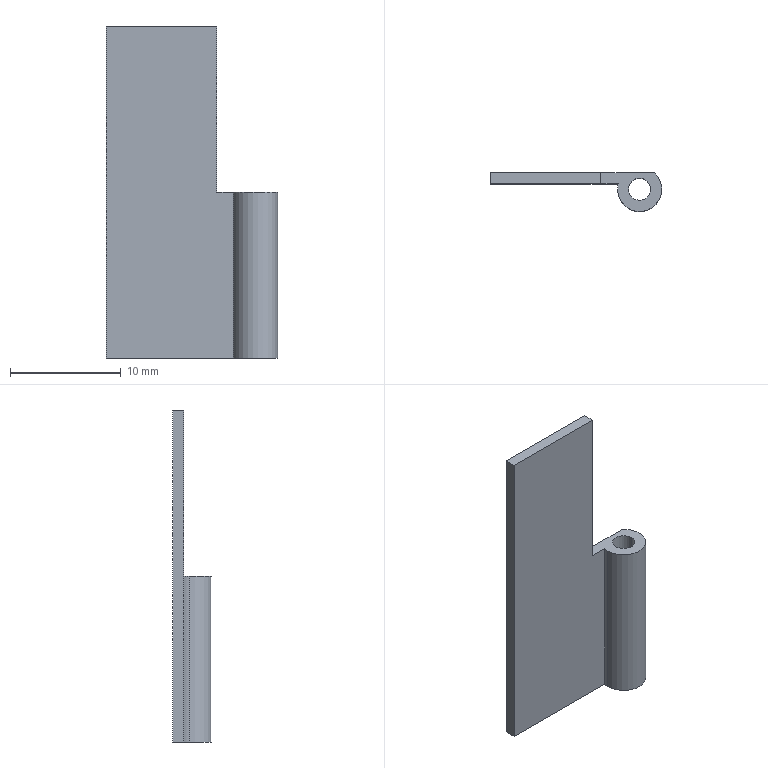Part | STEP file | Hinge leaf 1 | 1 solid | 12 faces | box 15.5 x 3.5 x 30 mm | volume 454.79 mm3 | plane 7 | cylinder 5 | commonest cylinder face diameters 4 x3 2 x2
STEP:
#1=CARTESIAN_POINT('',(0.,0.,0.));
#2=DIRECTION('',(0.,0.,1.));
#3=DIRECTION('',(1.,0.,0.));
#4=AXIS2_PLACEMENT_3D('',#1,#2,#3);
#5=CARTESIAN_POINT('',(15.5,-1.5,15.));
#6=VERTEX_POINT('',#5);
#7=CARTESIAN_POINT('',(14.823,0.,15.));
#8=VERTEX_POINT('',#7);
#9=CARTESIAN_POINT('',(13.5,-1.5,15.));
#10=DIRECTION('',(0.,0.,1.));
#11=DIRECTION('',(-1.,0.,0.));
#12=AXIS2_PLACEMENT_3D('',#9,#10,#11);
#13=CIRCLE('',#12,2.);
#14=CARTESIAN_POINT('',(13.5,-1.5,30.));
#15=DIRECTION('',(0.,0.,-1.));
#16=DIRECTION('',(-1.,0.,0.));
#17=AXIS2_PLACEMENT_3D('',#14,#15,#16);
#18=CYLINDRICAL_SURFACE('',#17,2.);
#19=CARTESIAN_POINT('',(6.283,15.));
#20=DIRECTION('',(-1.,0.));
#21=VECTOR('',#20,1.);
#22=LINE('',#19,#21);
#23=(GEOMETRIC_REPRESENTATION_CONTEXT(2)PARAMETRIC_REPRESENTATION_CONTEXT()REPRESENTATION_CONTEXT('',''));
#24=DEFINITIONAL_REPRESENTATION('',(#22),#23);
#25=PCURVE('',#18,#24);
#26=CARTESIAN_POINT('',(10.,-14.282,15.));
#27=DIRECTION('',(0.,0.,1.));
#28=DIRECTION('',(1.,0.,0.));
#29=AXIS2_PLACEMENT_3D('',#26,#27,#28);
#30=PLANE('',#29);
#31=CARTESIAN_POINT('',(3.5,12.782));
#32=DIRECTION('',(-1.,0.));
#33=AXIS2_PLACEMENT_2D('',#31,#32);
#34=CIRCLE('',#33,2.);
#35=(GEOMETRIC_REPRESENTATION_CONTEXT(2)PARAMETRIC_REPRESENTATION_CONTEXT()REPRESENTATION_CONTEXT('',''));
#36=DEFINITIONAL_REPRESENTATION('',(#34),#35);
#37=PCURVE('',#30,#36);
#38=SURFACE_CURVE('',#13,(#25,#37),.PCURVE_S1.);
#39=EDGE_CURVE('',#6,#8,#38,.T.);
#40=ORIENTED_EDGE('',*,*,#39,.F.);
#41=CARTESIAN_POINT('',(15.5,-1.5,0.));
#42=VERTEX_POINT('',#41);
#43=CARTESIAN_POINT('',(15.5,-1.5,30.));
#44=DIRECTION('',(0.,0.,-1.));
#45=VECTOR('',#44,1.);
#46=LINE('',#43,#45);
#47=CARTESIAN_POINT('',(3.142,0.));
#48=DIRECTION('',(0.,1.));
#49=VECTOR('',#48,1.);
#50=LINE('',#47,#49);
#51=(GEOMETRIC_REPRESENTATION_CONTEXT(2)PARAMETRIC_REPRESENTATION_CONTEXT()REPRESENTATION_CONTEXT('',''));
#52=DEFINITIONAL_REPRESENTATION('',(#50),#51);
#53=PCURVE('',#18,#52);
#54=CARTESIAN_POINT('',(13.5,-1.5,30.));
#55=DIRECTION('',(0.,0.,-1.));
#56=DIRECTION('',(-1.,0.,0.));
#57=AXIS2_PLACEMENT_3D('',#54,#55,#56);
#58=CYLINDRICAL_SURFACE('',#57,2.);
#59=CARTESIAN_POINT('',(3.142,0.));
#60=DIRECTION('',(0.,1.));
#61=VECTOR('',#60,1.);
#62=LINE('',#59,#61);
#63=(GEOMETRIC_REPRESENTATION_CONTEXT(2)PARAMETRIC_REPRESENTATION_CONTEXT()REPRESENTATION_CONTEXT('',''));
#64=DEFINITIONAL_REPRESENTATION('',(#62),#63);
#65=PCURVE('',#58,#64);
#66=SURFACE_CURVE('',#46,(#53,#65),.PCURVE_S1.);
#67=EDGE_CURVE('',#6,#42,#66,.T.);
#68=ORIENTED_EDGE('',*,*,#67,.T.);
#69=CARTESIAN_POINT('',(14.823,0.,0.));
#70=VERTEX_POINT('',#69);
#71=CARTESIAN_POINT('',(13.5,-1.5,0.));
#72=DIRECTION('',(0.,0.,1.));
#73=DIRECTION('',(-1.,0.,0.));
#74=AXIS2_PLACEMENT_3D('',#71,#72,#73);
#75=CIRCLE('',#74,2.);
#76=CARTESIAN_POINT('',(6.283,30.));
#77=DIRECTION('',(-1.,0.));
#78=VECTOR('',#77,1.);
#79=LINE('',#76,#78);
#80=(GEOMETRIC_REPRESENTATION_CONTEXT(2)PARAMETRIC_REPRESENTATION_CONTEXT()REPRESENTATION_CONTEXT('',''));
#81=DEFINITIONAL_REPRESENTATION('',(#79),#80);
#82=PCURVE('',#18,#81);
#83=CARTESIAN_POINT('',(13.5,-1.5,0.));
#84=DIRECTION('',(0.,0.,1.));
#85=DIRECTION('',(1.,0.,0.));
#86=AXIS2_PLACEMENT_3D('',#83,#84,#85);
#87=PLANE('',#86);
#88=CARTESIAN_POINT('',(0.,0.));
#89=DIRECTION('',(-1.,0.));
#90=AXIS2_PLACEMENT_2D('',#88,#89);
#91=CIRCLE('',#90,2.);
#92=(GEOMETRIC_REPRESENTATION_CONTEXT(2)PARAMETRIC_REPRESENTATION_CONTEXT()REPRESENTATION_CONTEXT('',''));
#93=DEFINITIONAL_REPRESENTATION('',(#91),#92);
#94=PCURVE('',#87,#93);
#95=SURFACE_CURVE('',#75,(#82,#94),.PCURVE_S1.);
#96=EDGE_CURVE('',#42,#70,#95,.T.);
#97=ORIENTED_EDGE('',*,*,#96,.T.);
#98=CARTESIAN_POINT('',(14.823,0.,30.));
#99=DIRECTION('',(0.,0.,1.));
#100=VECTOR('',#99,1.);
#101=LINE('',#98,#100);
#102=CARTESIAN_POINT('',(2.294,0.));
#103=DIRECTION('',(0.,-1.));
#104=VECTOR('',#103,1.);
#105=LINE('',#102,#104);
#106=(GEOMETRIC_REPRESENTATION_CONTEXT(2)PARAMETRIC_REPRESENTATION_CONTEXT()REPRESENTATION_CONTEXT('',''));
#107=DEFINITIONAL_REPRESENTATION('',(#105),#106);
#108=PCURVE('',#18,#107);
#109=CARTESIAN_POINT('',(0.,0.,30.));
#110=DIRECTION('',(0.,-1.,0.));
#111=DIRECTION('',(0.,0.,-1.));
#112=AXIS2_PLACEMENT_3D('',#109,#110,#111);
#113=PLANE('',#112);
#114=CARTESIAN_POINT('',(0.,14.823));
#115=DIRECTION('',(-1.,0.));
#116=VECTOR('',#115,1.);
#117=LINE('',#114,#116);
#118=(GEOMETRIC_REPRESENTATION_CONTEXT(2)PARAMETRIC_REPRESENTATION_CONTEXT()REPRESENTATION_CONTEXT('',''));
#119=DEFINITIONAL_REPRESENTATION('',(#117),#118);
#120=PCURVE('',#113,#119);
#121=SURFACE_CURVE('',#101,(#108,#120),.PCURVE_S1.);
#122=EDGE_CURVE('',#70,#8,#121,.T.);
#123=ORIENTED_EDGE('',*,*,#122,.T.);
#124=EDGE_LOOP('',(#40,#68,#97,#123));
#125=FACE_BOUND('',#124,.T.);
#126=ADVANCED_FACE('',(#125),#18,.T.);
#127=ORIENTED_EDGE('',*,*,#67,.F.);
#128=CARTESIAN_POINT('',(11.5,-1.5,15.));
#129=VERTEX_POINT('',#128);
#130=CARTESIAN_POINT('',(13.5,-1.5,15.));
#131=DIRECTION('',(0.,0.,1.));
#132=DIRECTION('',(-1.,0.,0.));
#133=AXIS2_PLACEMENT_3D('',#130,#131,#132);
#134=CIRCLE('',#133,2.);
#135=CARTESIAN_POINT('',(6.283,15.));
#136=DIRECTION('',(-1.,0.));
#137=VECTOR('',#136,1.);
#138=LINE('',#135,#137);
#139=(GEOMETRIC_REPRESENTATION_CONTEXT(2)PARAMETRIC_REPRESENTATION_CONTEXT()REPRESENTATION_CONTEXT('',''));
#140=DEFINITIONAL_REPRESENTATION('',(#138),#139);
#141=PCURVE('',#58,#140);
#142=CARTESIAN_POINT('',(3.5,12.782));
#143=DIRECTION('',(-1.,0.));
#144=AXIS2_PLACEMENT_2D('',#142,#143);
#145=CIRCLE('',#144,2.);
#146=(GEOMETRIC_REPRESENTATION_CONTEXT(2)PARAMETRIC_REPRESENTATION_CONTEXT()REPRESENTATION_CONTEXT('',''));
#147=DEFINITIONAL_REPRESENTATION('',(#145),#146);
#148=PCURVE('',#30,#147);
#149=SURFACE_CURVE('',#134,(#141,#148),.PCURVE_S1.);
#150=EDGE_CURVE('',#129,#6,#149,.T.);
#151=ORIENTED_EDGE('',*,*,#150,.F.);
#152=CARTESIAN_POINT('',(11.5,-1.5,0.));
#153=VERTEX_POINT('',#152);
#154=CARTESIAN_POINT('',(11.5,-1.5,30.));
#155=DIRECTION('',(0.,0.,-1.));
#156=VECTOR('',#155,1.);
#157=LINE('',#154,#156);
#158=CARTESIAN_POINT('',(6.283,0.));
#159=DIRECTION('',(0.,1.));
#160=VECTOR('',#159,1.);
#161=LINE('',#158,#160);
#162=(GEOMETRIC_REPRESENTATION_CONTEXT(2)PARAMETRIC_REPRESENTATION_CONTEXT()REPRESENTATION_CONTEXT('',''));
#163=DEFINITIONAL_REPRESENTATION('',(#161),#162);
#164=PCURVE('',#58,#163);
#165=CARTESIAN_POINT('',(13.5,-1.5,30.));
#166=DIRECTION('',(0.,0.,-1.));
#167=DIRECTION('',(-1.,0.,0.));
#168=AXIS2_PLACEMENT_3D('',#165,#166,#167);
#169=CYLINDRICAL_SURFACE('',#168,2.);
#170=CARTESIAN_POINT('',(0.,0.));
#171=DIRECTION('',(0.,1.));
#172=VECTOR('',#171,1.);
#173=LINE('',#170,#172);
#174=(GEOMETRIC_REPRESENTATION_CONTEXT(2)PARAMETRIC_REPRESENTATION_CONTEXT()REPRESENTATION_CONTEXT('',''));
#175=DEFINITIONAL_REPRESENTATION('',(#173),#174);
#176=PCURVE('',#169,#175);
#177=SURFACE_CURVE('',#157,(#164,#176),.PCURVE_S1.);
#178=EDGE_CURVE('',#129,#153,#177,.T.);
#179=ORIENTED_EDGE('',*,*,#178,.T.);
#180=CARTESIAN_POINT('',(13.5,-1.5,0.));
#181=DIRECTION('',(0.,0.,1.));
#182=DIRECTION('',(-1.,0.,0.));
#183=AXIS2_PLACEMENT_3D('',#180,#181,#182);
#184=CIRCLE('',#183,2.);
#185=CARTESIAN_POINT('',(6.283,30.));
#186=DIRECTION('',(-1.,0.));
#187=VECTOR('',#186,1.);
#188=LINE('',#185,#187);
#189=(GEOMETRIC_REPRESENTATION_CONTEXT(2)PARAMETRIC_REPRESENTATION_CONTEXT()REPRESENTATION_CONTEXT('',''));
#190=DEFINITIONAL_REPRESENTATION('',(#188),#189);
#191=PCURVE('',#58,#190);
#192=CARTESIAN_POINT('',(0.,0.));
#193=DIRECTION('',(-1.,0.));
#194=AXIS2_PLACEMENT_2D('',#192,#193);
#195=CIRCLE('',#194,2.);
#196=(GEOMETRIC_REPRESENTATION_CONTEXT(2)PARAMETRIC_REPRESENTATION_CONTEXT()REPRESENTATION_CONTEXT('',''));
#197=DEFINITIONAL_REPRESENTATION('',(#195),#196);
#198=PCURVE('',#87,#197);
#199=SURFACE_CURVE('',#184,(#191,#198),.PCURVE_S1.);
#200=EDGE_CURVE('',#153,#42,#199,.T.);
#201=ORIENTED_EDGE('',*,*,#200,.T.);
#202=EDGE_LOOP('',(#127,#151,#179,#201));
#203=FACE_BOUND('',#202,.T.);
#204=ADVANCED_FACE('',(#203),#58,.T.);
#205=CARTESIAN_POINT('',(12.5,-1.5,15.));
#206=VERTEX_POINT('',#205);
#207=CARTESIAN_POINT('',(12.5,-1.5,0.));
#208=VERTEX_POINT('',#207);
#209=CARTESIAN_POINT('',(12.5,-1.5,30.));
#210=DIRECTION('',(0.,0.,-1.));
#211=VECTOR('',#210,1.);
#212=LINE('',#209,#211);
#213=CARTESIAN_POINT('',(13.5,-1.5,30.));
#214=DIRECTION('',(0.,0.,-1.));
#215=DIRECTION('',(-1.,0.,0.));
#216=AXIS2_PLACEMENT_3D('',#213,#214,#215);
#217=CYLINDRICAL_SURFACE('',#216,1.);
#218=CARTESIAN_POINT('',(6.283,0.));
#219=DIRECTION('',(0.,1.));
#220=VECTOR('',#219,1.);
#221=LINE('',#218,#220);
#222=(GEOMETRIC_REPRESENTATION_CONTEXT(2)PARAMETRIC_REPRESENTATION_CONTEXT()REPRESENTATION_CONTEXT('',''));
#223=DEFINITIONAL_REPRESENTATION('',(#221),#222);
#224=PCURVE('',#217,#223);
#225=CARTESIAN_POINT('',(13.5,-1.5,30.));
#226=DIRECTION('',(0.,0.,-1.));
#227=DIRECTION('',(-1.,0.,0.));
#228=AXIS2_PLACEMENT_3D('',#225,#226,#227);
#229=CYLINDRICAL_SURFACE('',#228,1.);
#230=CARTESIAN_POINT('',(0.,0.));
#231=DIRECTION('',(0.,1.));
#232=VECTOR('',#231,1.);
#233=LINE('',#230,#232);
#234=(GEOMETRIC_REPRESENTATION_CONTEXT(2)PARAMETRIC_REPRESENTATION_CONTEXT()REPRESENTATION_CONTEXT('',''));
#235=DEFINITIONAL_REPRESENTATION('',(#233),#234);
#236=PCURVE('',#229,#235);
#237=SURFACE_CURVE('',#212,(#224,#236),.PCURVE_S1.);
#238=EDGE_CURVE('',#206,#208,#237,.T.);
#239=ORIENTED_EDGE('',*,*,#238,.T.);
#240=CARTESIAN_POINT('',(14.5,-1.5,0.));
#241=VERTEX_POINT('',#240);
#242=CARTESIAN_POINT('',(13.5,-1.5,0.));
#243=DIRECTION('',(0.,0.,-1.));
#244=DIRECTION('',(-1.,0.,0.));
#245=AXIS2_PLACEMENT_3D('',#242,#243,#244);
#246=CIRCLE('',#245,1.);
#247=CARTESIAN_POINT('',(0.,30.));
#248=DIRECTION('',(1.,0.));
#249=VECTOR('',#248,1.);
#250=LINE('',#247,#249);
#251=(GEOMETRIC_REPRESENTATION_CONTEXT(2)PARAMETRIC_REPRESENTATION_CONTEXT()REPRESENTATION_CONTEXT('',''));
#252=DEFINITIONAL_REPRESENTATION('',(#250),#251);
#253=PCURVE('',#217,#252);
#254=CARTESIAN_POINT('',(-1.,0.));
#255=CARTESIAN_POINT('',(-1.,1.732));
#256=CARTESIAN_POINT('',(0.5,0.866));
#257=CARTESIAN_POINT('',(2.,0.));
#258=CARTESIAN_POINT('',(0.5,-0.866));
#259=CARTESIAN_POINT('',(-1.,-1.732));
#260=CARTESIAN_POINT('',(-1.,0.));
#261=(BOUNDED_CURVE()B_SPLINE_CURVE(2,(#254,#255,#256,#257,#258,#259,#260),.UNSPECIFIED.,.T.,.F.)B_SPLINE_CURVE_WITH_KNOTS((1,2,2,2,2,1),(-2.094,0.,2.094,4.189,6.283,8.378),.UNSPECIFIED.)CURVE()GEOMETRIC_REPRESENTATION_ITEM()RATIONAL_B_SPLINE_CURVE((1.,0.5,1.,0.5,1.,0.5,1.))REPRESENTATION_ITEM(''));
#262=(GEOMETRIC_REPRESENTATION_CONTEXT(2)PARAMETRIC_REPRESENTATION_CONTEXT()REPRESENTATION_CONTEXT('',''));
#263=DEFINITIONAL_REPRESENTATION('',(#261),#262);
#264=PCURVE('',#87,#263);
#265=SURFACE_CURVE('',#246,(#253,#264),.PCURVE_S1.);
#266=EDGE_CURVE('',#241,#208,#265,.T.);
#267=ORIENTED_EDGE('',*,*,#266,.F.);
#268=CARTESIAN_POINT('',(14.5,-1.5,15.));
#269=VERTEX_POINT('',#268);
#270=CARTESIAN_POINT('',(14.5,-1.5,30.));
#271=DIRECTION('',(0.,0.,-1.));
#272=VECTOR('',#271,1.);
#273=LINE('',#270,#272);
#274=CARTESIAN_POINT('',(3.142,0.));
#275=DIRECTION('',(0.,1.));
#276=VECTOR('',#275,1.);
#277=LINE('',#274,#276);
#278=(GEOMETRIC_REPRESENTATION_CONTEXT(2)PARAMETRIC_REPRESENTATION_CONTEXT()REPRESENTATION_CONTEXT('',''));
#279=DEFINITIONAL_REPRESENTATION('',(#277),#278);
#280=PCURVE('',#217,#279);
#281=CARTESIAN_POINT('',(3.142,0.));
#282=DIRECTION('',(0.,1.));
#283=VECTOR('',#282,1.);
#284=LINE('',#281,#283);
#285=(GEOMETRIC_REPRESENTATION_CONTEXT(2)PARAMETRIC_REPRESENTATION_CONTEXT()REPRESENTATION_CONTEXT('',''));
#286=DEFINITIONAL_REPRESENTATION('',(#284),#285);
#287=PCURVE('',#229,#286);
#288=SURFACE_CURVE('',#273,(#280,#287),.PCURVE_S1.);
#289=EDGE_CURVE('',#269,#241,#288,.T.);
#290=ORIENTED_EDGE('',*,*,#289,.F.);
#291=CARTESIAN_POINT('',(13.5,-1.5,15.));
#292=DIRECTION('',(0.,0.,-1.));
#293=DIRECTION('',(-1.,0.,0.));
#294=AXIS2_PLACEMENT_3D('',#291,#292,#293);
#295=CIRCLE('',#294,1.);
#296=CARTESIAN_POINT('',(0.,15.));
#297=DIRECTION('',(1.,0.));
#298=VECTOR('',#297,1.);
#299=LINE('',#296,#298);
#300=(GEOMETRIC_REPRESENTATION_CONTEXT(2)PARAMETRIC_REPRESENTATION_CONTEXT()REPRESENTATION_CONTEXT('',''));
#301=DEFINITIONAL_REPRESENTATION('',(#299),#300);
#302=PCURVE('',#217,#301);
#303=CARTESIAN_POINT('',(2.5,12.782));
#304=CARTESIAN_POINT('',(2.5,14.514));
#305=CARTESIAN_POINT('',(4.,13.648));
#306=CARTESIAN_POINT('',(5.5,12.782));
#307=CARTESIAN_POINT('',(4.,11.916));
#308=CARTESIAN_POINT('',(2.5,11.05));
#309=CARTESIAN_POINT('',(2.5,12.782));
#310=(BOUNDED_CURVE()B_SPLINE_CURVE(2,(#303,#304,#305,#306,#307,#308,#309),.UNSPECIFIED.,.T.,.F.)B_SPLINE_CURVE_WITH_KNOTS((1,2,2,2,2,1),(-2.094,0.,2.094,4.189,6.283,8.378),.UNSPECIFIED.)CURVE()GEOMETRIC_REPRESENTATION_ITEM()RATIONAL_B_SPLINE_CURVE((1.,0.5,1.,0.5,1.,0.5,1.))REPRESENTATION_ITEM(''));
#311=(GEOMETRIC_REPRESENTATION_CONTEXT(2)PARAMETRIC_REPRESENTATION_CONTEXT()REPRESENTATION_CONTEXT('',''));
#312=DEFINITIONAL_REPRESENTATION('',(#310),#311);
#313=PCURVE('',#30,#312);
#314=SURFACE_CURVE('',#295,(#302,#313),.PCURVE_S1.);
#315=EDGE_CURVE('',#269,#206,#314,.T.);
#316=ORIENTED_EDGE('',*,*,#315,.T.);
#317=EDGE_LOOP('',(#239,#267,#290,#316));
#318=FACE_BOUND('',#317,.F.);
#319=ADVANCED_FACE('',(#318),#217,.F.);
#320=CARTESIAN_POINT('',(10.,0.,15.));
#321=VERTEX_POINT('',#320);
#322=CARTESIAN_POINT('',(10.,0.,30.));
#323=VERTEX_POINT('',#322);
#324=CARTESIAN_POINT('',(10.,0.,30.));
#325=DIRECTION('',(0.,0.,1.));
#326=VECTOR('',#325,1.);
#327=LINE('',#324,#326);
#328=CARTESIAN_POINT('',(0.,10.));
#329=DIRECTION('',(-1.,0.));
#330=VECTOR('',#329,1.);
#331=LINE('',#328,#330);
#332=(GEOMETRIC_REPRESENTATION_CONTEXT(2)PARAMETRIC_REPRESENTATION_CONTEXT()REPRESENTATION_CONTEXT('',''));
#333=DEFINITIONAL_REPRESENTATION('',(#331),#332);
#334=PCURVE('',#113,#333);
#335=CARTESIAN_POINT('',(10.,2.063,15.));
#336=DIRECTION('',(-1.,0.,0.));
#337=DIRECTION('',(0.,-1.,0.));
#338=AXIS2_PLACEMENT_3D('',#335,#336,#337);
#339=PLANE('',#338);
#340=CARTESIAN_POINT('',(2.063,15.));
#341=DIRECTION('',(0.,1.));
#342=VECTOR('',#341,1.);
#343=LINE('',#340,#342);
#344=(GEOMETRIC_REPRESENTATION_CONTEXT(2)PARAMETRIC_REPRESENTATION_CONTEXT()REPRESENTATION_CONTEXT('',''));
#345=DEFINITIONAL_REPRESENTATION('',(#343),#344);
#346=PCURVE('',#339,#345);
#347=SURFACE_CURVE('',#327,(#334,#346),.PCURVE_S1.);
#348=EDGE_CURVE('',#321,#323,#347,.T.);
#349=ORIENTED_EDGE('',*,*,#348,.F.);
#350=CARTESIAN_POINT('',(0.,0.,15.));
#351=DIRECTION('',(-1.,0.,0.));
#352=VECTOR('',#351,1.);
#353=LINE('',#350,#352);
#354=CARTESIAN_POINT('',(15.,0.));
#355=DIRECTION('',(0.,-1.));
#356=VECTOR('',#355,1.);
#357=LINE('',#354,#356);
#358=(GEOMETRIC_REPRESENTATION_CONTEXT(2)PARAMETRIC_REPRESENTATION_CONTEXT()REPRESENTATION_CONTEXT('',''));
#359=DEFINITIONAL_REPRESENTATION('',(#357),#358);
#360=PCURVE('',#113,#359);
#361=CARTESIAN_POINT('',(-10.,14.282));
#362=DIRECTION('',(-1.,0.));
#363=VECTOR('',#362,1.);
#364=LINE('',#361,#363);
#365=(GEOMETRIC_REPRESENTATION_CONTEXT(2)PARAMETRIC_REPRESENTATION_CONTEXT()REPRESENTATION_CONTEXT('',''));
#366=DEFINITIONAL_REPRESENTATION('',(#364),#365);
#367=PCURVE('',#30,#366);
#368=SURFACE_CURVE('',#353,(#360,#367),.PCURVE_S1.);
#369=EDGE_CURVE('',#8,#321,#368,.T.);
#370=ORIENTED_EDGE('',*,*,#369,.F.);
#371=ORIENTED_EDGE('',*,*,#122,.F.);
#372=CARTESIAN_POINT('',(0.,0.,0.));
#373=VERTEX_POINT('',#372);
#374=CARTESIAN_POINT('',(0.,0.,0.));
#375=DIRECTION('',(1.,0.,0.));
#376=VECTOR('',#375,1.);
#377=LINE('',#374,#376);
#378=CARTESIAN_POINT('',(30.,0.));
#379=DIRECTION('',(0.,1.));
#380=VECTOR('',#379,1.);
#381=LINE('',#378,#380);
#382=(GEOMETRIC_REPRESENTATION_CONTEXT(2)PARAMETRIC_REPRESENTATION_CONTEXT()REPRESENTATION_CONTEXT('',''));
#383=DEFINITIONAL_REPRESENTATION('',(#381),#382);
#384=PCURVE('',#113,#383);
#385=CARTESIAN_POINT('',(-13.5,1.5));
#386=DIRECTION('',(1.,0.));
#387=VECTOR('',#386,1.);
#388=LINE('',#385,#387);
#389=(GEOMETRIC_REPRESENTATION_CONTEXT(2)PARAMETRIC_REPRESENTATION_CONTEXT()REPRESENTATION_CONTEXT('',''));
#390=DEFINITIONAL_REPRESENTATION('',(#388),#389);
#391=PCURVE('',#87,#390);
#392=SURFACE_CURVE('',#377,(#384,#391),.PCURVE_S1.);
#393=EDGE_CURVE('',#373,#70,#392,.T.);
#394=ORIENTED_EDGE('',*,*,#393,.F.);
#395=CARTESIAN_POINT('',(0.,0.,30.));
#396=VERTEX_POINT('',#395);
#397=CARTESIAN_POINT('',(0.,0.,30.));
#398=DIRECTION('',(0.,0.,-1.));
#399=VECTOR('',#398,1.);
#400=LINE('',#397,#399);
#401=CARTESIAN_POINT('',(0.,0.));
#402=DIRECTION('',(1.,0.));
#403=VECTOR('',#402,1.);
#404=LINE('',#401,#403);
#405=(GEOMETRIC_REPRESENTATION_CONTEXT(2)PARAMETRIC_REPRESENTATION_CONTEXT()REPRESENTATION_CONTEXT('',''));
#406=DEFINITIONAL_REPRESENTATION('',(#404),#405);
#407=PCURVE('',#113,#406);
#408=CARTESIAN_POINT('',(0.,0.,30.));
#409=DIRECTION('',(1.,0.,0.));
#410=DIRECTION('',(0.,1.,0.));
#411=AXIS2_PLACEMENT_3D('',#408,#409,#410);
#412=PLANE('',#411);
#413=CARTESIAN_POINT('',(0.,0.));
#414=DIRECTION('',(0.,-1.));
#415=VECTOR('',#414,1.);
#416=LINE('',#413,#415);
#417=(GEOMETRIC_REPRESENTATION_CONTEXT(2)PARAMETRIC_REPRESENTATION_CONTEXT()REPRESENTATION_CONTEXT('',''));
#418=DEFINITIONAL_REPRESENTATION('',(#416),#417);
#419=PCURVE('',#412,#418);
#420=SURFACE_CURVE('',#400,(#407,#419),.PCURVE_S1.);
#421=EDGE_CURVE('',#396,#373,#420,.T.);
#422=ORIENTED_EDGE('',*,*,#421,.F.);
#423=CARTESIAN_POINT('',(0.,0.,30.));
#424=DIRECTION('',(-1.,0.,0.));
#425=VECTOR('',#424,1.);
#426=LINE('',#423,#425);
#427=CARTESIAN_POINT('',(0.,0.));
#428=DIRECTION('',(0.,-1.));
#429=VECTOR('',#428,1.);
#430=LINE('',#427,#429);
#431=(GEOMETRIC_REPRESENTATION_CONTEXT(2)PARAMETRIC_REPRESENTATION_CONTEXT()REPRESENTATION_CONTEXT('',''));
#432=DEFINITIONAL_REPRESENTATION('',(#430),#431);
#433=PCURVE('',#113,#432);
#434=CARTESIAN_POINT('',(13.5,-1.5,30.));
#435=DIRECTION('',(0.,0.,1.));
#436=DIRECTION('',(1.,0.,0.));
#437=AXIS2_PLACEMENT_3D('',#434,#435,#436);
#438=PLANE('',#437);
#439=CARTESIAN_POINT('',(-13.5,1.5));
#440=DIRECTION('',(-1.,0.));
#441=VECTOR('',#440,1.);
#442=LINE('',#439,#441);
#443=(GEOMETRIC_REPRESENTATION_CONTEXT(2)PARAMETRIC_REPRESENTATION_CONTEXT()REPRESENTATION_CONTEXT('',''));
#444=DEFINITIONAL_REPRESENTATION('',(#442),#443);
#445=PCURVE('',#438,#444);
#446=SURFACE_CURVE('',#426,(#433,#445),.PCURVE_S1.);
#447=EDGE_CURVE('',#323,#396,#446,.T.);
#448=ORIENTED_EDGE('',*,*,#447,.F.);
#449=EDGE_LOOP('',(#349,#370,#371,#394,#422,#448));
#450=FACE_BOUND('',#449,.T.);
#451=ADVANCED_FACE('',(#450),#113,.F.);
#452=CARTESIAN_POINT('',(0.,-1.,30.));
#453=VERTEX_POINT('',#452);
#454=CARTESIAN_POINT('',(0.,-1.5,30.));
#455=DIRECTION('',(0.,-1.,0.));
#456=VECTOR('',#455,1.);
#457=LINE('',#454,#456);
#458=CARTESIAN_POINT('',(-13.5,0.));
#459=DIRECTION('',(0.,-1.));
#460=VECTOR('',#459,1.);
#461=LINE('',#458,#460);
#462=(GEOMETRIC_REPRESENTATION_CONTEXT(2)PARAMETRIC_REPRESENTATION_CONTEXT()REPRESENTATION_CONTEXT('',''));
#463=DEFINITIONAL_REPRESENTATION('',(#461),#462);
#464=PCURVE('',#438,#463);
#465=CARTESIAN_POINT('',(-1.5,0.));
#466=DIRECTION('',(-1.,0.));
#467=VECTOR('',#466,1.);
#468=LINE('',#465,#467);
#469=(GEOMETRIC_REPRESENTATION_CONTEXT(2)PARAMETRIC_REPRESENTATION_CONTEXT()REPRESENTATION_CONTEXT('',''));
#470=DEFINITIONAL_REPRESENTATION('',(#468),#469);
#471=PCURVE('',#412,#470);
#472=SURFACE_CURVE('',#457,(#464,#471),.PCURVE_S1.);
#473=EDGE_CURVE('',#396,#453,#472,.T.);
#474=ORIENTED_EDGE('',*,*,#473,.T.);
#475=CARTESIAN_POINT('',(10.,-1.,30.));
#476=VERTEX_POINT('',#475);
#477=CARTESIAN_POINT('',(13.5,-1.,30.));
#478=DIRECTION('',(1.,0.,0.));
#479=VECTOR('',#478,1.);
#480=LINE('',#477,#479);
#481=CARTESIAN_POINT('',(0.,0.5));
#482=DIRECTION('',(1.,0.));
#483=VECTOR('',#482,1.);
#484=LINE('',#481,#483);
#485=(GEOMETRIC_REPRESENTATION_CONTEXT(2)PARAMETRIC_REPRESENTATION_CONTEXT()REPRESENTATION_CONTEXT('',''));
#486=DEFINITIONAL_REPRESENTATION('',(#484),#485);
#487=PCURVE('',#438,#486);
#488=CARTESIAN_POINT('',(0.,-1.,30.));
#489=DIRECTION('',(0.,1.,0.));
#490=DIRECTION('',(-1.,0.,0.));
#491=AXIS2_PLACEMENT_3D('',#488,#489,#490);
#492=PLANE('',#491);
#493=CARTESIAN_POINT('',(-13.5,0.));
#494=DIRECTION('',(-1.,0.));
#495=VECTOR('',#494,1.);
#496=LINE('',#493,#495);
#497=(GEOMETRIC_REPRESENTATION_CONTEXT(2)PARAMETRIC_REPRESENTATION_CONTEXT()REPRESENTATION_CONTEXT('',''));
#498=DEFINITIONAL_REPRESENTATION('',(#496),#497);
#499=PCURVE('',#492,#498);
#500=SURFACE_CURVE('',#480,(#487,#499),.PCURVE_S1.);
#501=EDGE_CURVE('',#453,#476,#500,.T.);
#502=ORIENTED_EDGE('',*,*,#501,.T.);
#503=CARTESIAN_POINT('',(10.,-1.5,30.));
#504=DIRECTION('',(0.,1.,0.));
#505=VECTOR('',#504,1.);
#506=LINE('',#503,#505);
#507=CARTESIAN_POINT('',(-3.5,0.));
#508=DIRECTION('',(0.,1.));
#509=VECTOR('',#508,1.);
#510=LINE('',#507,#509);
#511=(GEOMETRIC_REPRESENTATION_CONTEXT(2)PARAMETRIC_REPRESENTATION_CONTEXT()REPRESENTATION_CONTEXT('',''));
#512=DEFINITIONAL_REPRESENTATION('',(#510),#511);
#513=PCURVE('',#438,#512);
#514=CARTESIAN_POINT('',(3.563,15.));
#515=DIRECTION('',(-1.,0.));
#516=VECTOR('',#515,1.);
#517=LINE('',#514,#516);
#518=(GEOMETRIC_REPRESENTATION_CONTEXT(2)PARAMETRIC_REPRESENTATION_CONTEXT()REPRESENTATION_CONTEXT('',''));
#519=DEFINITIONAL_REPRESENTATION('',(#517),#518);
#520=PCURVE('',#339,#519);
#521=SURFACE_CURVE('',#506,(#513,#520),.PCURVE_S1.);
#522=EDGE_CURVE('',#476,#323,#521,.T.);
#523=ORIENTED_EDGE('',*,*,#522,.T.);
#524=ORIENTED_EDGE('',*,*,#447,.T.);
#525=EDGE_LOOP('',(#474,#502,#523,#524));
#526=FACE_BOUND('',#525,.T.);
#527=ADVANCED_FACE('',(#526),#438,.T.);
#528=CARTESIAN_POINT('',(10.,-1.,15.));
#529=VERTEX_POINT('',#528);
#530=CARTESIAN_POINT('',(10.,-1.,15.));
#531=DIRECTION('',(0.,0.,1.));
#532=VECTOR('',#531,1.);
#533=LINE('',#530,#532);
#534=CARTESIAN_POINT('',(3.063,0.));
#535=DIRECTION('',(0.,1.));
#536=VECTOR('',#535,1.);
#537=LINE('',#534,#536);
#538=(GEOMETRIC_REPRESENTATION_CONTEXT(2)PARAMETRIC_REPRESENTATION_CONTEXT()REPRESENTATION_CONTEXT('',''));
#539=DEFINITIONAL_REPRESENTATION('',(#537),#538);
#540=PCURVE('',#339,#539);
#541=CARTESIAN_POINT('',(-10.,-15.));
#542=DIRECTION('',(0.,1.));
#543=VECTOR('',#542,1.);
#544=LINE('',#541,#543);
#545=(GEOMETRIC_REPRESENTATION_CONTEXT(2)PARAMETRIC_REPRESENTATION_CONTEXT()REPRESENTATION_CONTEXT('',''));
#546=DEFINITIONAL_REPRESENTATION('',(#544),#545);
#547=PCURVE('',#492,#546);
#548=SURFACE_CURVE('',#533,(#540,#547),.PCURVE_S1.);
#549=EDGE_CURVE('',#529,#476,#548,.T.);
#550=ORIENTED_EDGE('',*,*,#549,.F.);
#551=CARTESIAN_POINT('',(10.,2.063,15.));
#552=DIRECTION('',(0.,-1.,0.));
#553=VECTOR('',#552,1.);
#554=LINE('',#551,#553);
#555=CARTESIAN_POINT('',(0.,0.));
#556=DIRECTION('',(1.,0.));
#557=VECTOR('',#556,1.);
#558=LINE('',#555,#557);
#559=(GEOMETRIC_REPRESENTATION_CONTEXT(2)PARAMETRIC_REPRESENTATION_CONTEXT()REPRESENTATION_CONTEXT('',''));
#560=DEFINITIONAL_REPRESENTATION('',(#558),#559);
#561=PCURVE('',#339,#560);
#562=CARTESIAN_POINT('',(0.,16.345));
#563=DIRECTION('',(0.,-1.));
#564=VECTOR('',#563,1.);
#565=LINE('',#562,#564);
#566=(GEOMETRIC_REPRESENTATION_CONTEXT(2)PARAMETRIC_REPRESENTATION_CONTEXT()REPRESENTATION_CONTEXT('',''));
#567=DEFINITIONAL_REPRESENTATION('',(#565),#566);
#568=PCURVE('',#30,#567);
#569=SURFACE_CURVE('',#554,(#561,#568),.PCURVE_S1.);
#570=EDGE_CURVE('',#321,#529,#569,.T.);
#571=ORIENTED_EDGE('',*,*,#570,.F.);
#572=ORIENTED_EDGE('',*,*,#348,.T.);
#573=ORIENTED_EDGE('',*,*,#522,.F.);
#574=EDGE_LOOP('',(#550,#571,#572,#573));
#575=FACE_BOUND('',#574,.T.);
#576=ADVANCED_FACE('',(#575),#339,.F.);
#577=CARTESIAN_POINT('',(11.564,-1.,15.));
#578=VERTEX_POINT('',#577);
#579=CARTESIAN_POINT('',(10.,-1.,15.));
#580=DIRECTION('',(1.,0.,0.));
#581=VECTOR('',#580,1.);
#582=LINE('',#579,#581);
#583=CARTESIAN_POINT('',(0.,13.282));
#584=DIRECTION('',(1.,0.));
#585=VECTOR('',#584,1.);
#586=LINE('',#583,#585);
#587=(GEOMETRIC_REPRESENTATION_CONTEXT(2)PARAMETRIC_REPRESENTATION_CONTEXT()REPRESENTATION_CONTEXT('',''));
#588=DEFINITIONAL_REPRESENTATION('',(#586),#587);
#589=PCURVE('',#30,#588);
#590=CARTESIAN_POINT('',(-10.,-15.));
#591=DIRECTION('',(-1.,0.));
#592=VECTOR('',#591,1.);
#593=LINE('',#590,#592);
#594=(GEOMETRIC_REPRESENTATION_CONTEXT(2)PARAMETRIC_REPRESENTATION_CONTEXT()REPRESENTATION_CONTEXT('',''));
#595=DEFINITIONAL_REPRESENTATION('',(#593),#594);
#596=PCURVE('',#492,#595);
#597=SURFACE_CURVE('',#582,(#589,#596),.PCURVE_S1.);
#598=EDGE_CURVE('',#529,#578,#597,.T.);
#599=ORIENTED_EDGE('',*,*,#598,.T.);
#600=CARTESIAN_POINT('',(13.5,-1.5,15.));
#601=DIRECTION('',(0.,0.,1.));
#602=DIRECTION('',(-1.,0.,0.));
#603=AXIS2_PLACEMENT_3D('',#600,#601,#602);
#604=CIRCLE('',#603,2.);
#605=CARTESIAN_POINT('',(3.5,12.782));
#606=DIRECTION('',(-1.,0.));
#607=AXIS2_PLACEMENT_2D('',#605,#606);
#608=CIRCLE('',#607,2.);
#609=(GEOMETRIC_REPRESENTATION_CONTEXT(2)PARAMETRIC_REPRESENTATION_CONTEXT()REPRESENTATION_CONTEXT('',''));
#610=DEFINITIONAL_REPRESENTATION('',(#608),#609);
#611=PCURVE('',#30,#610);
#612=CARTESIAN_POINT('',(6.283,15.));
#613=DIRECTION('',(-1.,0.));
#614=VECTOR('',#613,1.);
#615=LINE('',#612,#614);
#616=(GEOMETRIC_REPRESENTATION_CONTEXT(2)PARAMETRIC_REPRESENTATION_CONTEXT()REPRESENTATION_CONTEXT('',''));
#617=DEFINITIONAL_REPRESENTATION('',(#615),#616);
#618=PCURVE('',#169,#617);
#619=SURFACE_CURVE('',#604,(#611,#618),.PCURVE_S1.);
#620=EDGE_CURVE('',#578,#129,#619,.T.);
#621=ORIENTED_EDGE('',*,*,#620,.T.);
#622=ORIENTED_EDGE('',*,*,#150,.T.);
#623=ORIENTED_EDGE('',*,*,#39,.T.);
#624=ORIENTED_EDGE('',*,*,#369,.T.);
#625=ORIENTED_EDGE('',*,*,#570,.T.);
#626=EDGE_LOOP('',(#599,#621,#622,#623,#624,#625));
#627=FACE_BOUND('',#626,.T.);
#628=CARTESIAN_POINT('',(13.5,-1.5,15.));
#629=DIRECTION('',(0.,0.,-1.));
#630=DIRECTION('',(-1.,0.,0.));
#631=AXIS2_PLACEMENT_3D('',#628,#629,#630);
#632=CIRCLE('',#631,1.);
#633=CARTESIAN_POINT('',(2.5,12.782));
#634=CARTESIAN_POINT('',(2.5,14.514));
#635=CARTESIAN_POINT('',(4.,13.648));
#636=CARTESIAN_POINT('',(5.5,12.782));
#637=CARTESIAN_POINT('',(4.,11.916));
#638=CARTESIAN_POINT('',(2.5,11.05));
#639=CARTESIAN_POINT('',(2.5,12.782));
#640=(BOUNDED_CURVE()B_SPLINE_CURVE(2,(#633,#634,#635,#636,#637,#638,#639),.UNSPECIFIED.,.T.,.F.)B_SPLINE_CURVE_WITH_KNOTS((1,2,2,2,2,1),(-2.094,0.,2.094,4.189,6.283,8.378),.UNSPECIFIED.)CURVE()GEOMETRIC_REPRESENTATION_ITEM()RATIONAL_B_SPLINE_CURVE((1.,0.5,1.,0.5,1.,0.5,1.))REPRESENTATION_ITEM(''));
#641=(GEOMETRIC_REPRESENTATION_CONTEXT(2)PARAMETRIC_REPRESENTATION_CONTEXT()REPRESENTATION_CONTEXT('',''));
#642=DEFINITIONAL_REPRESENTATION('',(#640),#641);
#643=PCURVE('',#30,#642);
#644=CARTESIAN_POINT('',(0.,15.));
#645=DIRECTION('',(1.,0.));
#646=VECTOR('',#645,1.);
#647=LINE('',#644,#646);
#648=(GEOMETRIC_REPRESENTATION_CONTEXT(2)PARAMETRIC_REPRESENTATION_CONTEXT()REPRESENTATION_CONTEXT('',''));
#649=DEFINITIONAL_REPRESENTATION('',(#647),#648);
#650=PCURVE('',#229,#649);
#651=SURFACE_CURVE('',#632,(#643,#650),.PCURVE_S1.);
#652=EDGE_CURVE('',#206,#269,#651,.T.);
#653=ORIENTED_EDGE('',*,*,#652,.T.);
#654=ORIENTED_EDGE('',*,*,#315,.T.);
#655=EDGE_LOOP('',(#653,#654));
#656=FACE_BOUND('',#655,.T.);
#657=ADVANCED_FACE('',(#627,#656),#30,.T.);
#658=ORIENTED_EDGE('',*,*,#178,.F.);
#659=ORIENTED_EDGE('',*,*,#620,.F.);
#660=CARTESIAN_POINT('',(11.564,-1.,0.));
#661=VERTEX_POINT('',#660);
#662=CARTESIAN_POINT('',(11.564,-1.,30.));
#663=DIRECTION('',(0.,0.,-1.));
#664=VECTOR('',#663,1.);
#665=LINE('',#662,#664);
#666=CARTESIAN_POINT('',(0.2527,0.));
#667=DIRECTION('',(0.,1.));
#668=VECTOR('',#667,1.);
#669=LINE('',#666,#668);
#670=(GEOMETRIC_REPRESENTATION_CONTEXT(2)PARAMETRIC_REPRESENTATION_CONTEXT()REPRESENTATION_CONTEXT('',''));
#671=DEFINITIONAL_REPRESENTATION('',(#669),#670);
#672=PCURVE('',#169,#671);
#673=CARTESIAN_POINT('',(-11.564,0.));
#674=DIRECTION('',(0.,-1.));
#675=VECTOR('',#674,1.);
#676=LINE('',#673,#675);
#677=(GEOMETRIC_REPRESENTATION_CONTEXT(2)PARAMETRIC_REPRESENTATION_CONTEXT()REPRESENTATION_CONTEXT('',''));
#678=DEFINITIONAL_REPRESENTATION('',(#676),#677);
#679=PCURVE('',#492,#678);
#680=SURFACE_CURVE('',#665,(#672,#679),.PCURVE_S1.);
#681=EDGE_CURVE('',#578,#661,#680,.T.);
#682=ORIENTED_EDGE('',*,*,#681,.T.);
#683=CARTESIAN_POINT('',(13.5,-1.5,0.));
#684=DIRECTION('',(0.,0.,1.));
#685=DIRECTION('',(-1.,0.,0.));
#686=AXIS2_PLACEMENT_3D('',#683,#684,#685);
#687=CIRCLE('',#686,2.);
#688=CARTESIAN_POINT('',(6.283,30.));
#689=DIRECTION('',(-1.,0.));
#690=VECTOR('',#689,1.);
#691=LINE('',#688,#690);
#692=(GEOMETRIC_REPRESENTATION_CONTEXT(2)PARAMETRIC_REPRESENTATION_CONTEXT()REPRESENTATION_CONTEXT('',''));
#693=DEFINITIONAL_REPRESENTATION('',(#691),#692);
#694=PCURVE('',#169,#693);
#695=CARTESIAN_POINT('',(0.,0.));
#696=DIRECTION('',(-1.,0.));
#697=AXIS2_PLACEMENT_2D('',#695,#696);
#698=CIRCLE('',#697,2.);
#699=(GEOMETRIC_REPRESENTATION_CONTEXT(2)PARAMETRIC_REPRESENTATION_CONTEXT()REPRESENTATION_CONTEXT('',''));
#700=DEFINITIONAL_REPRESENTATION('',(#698),#699);
#701=PCURVE('',#87,#700);
#702=SURFACE_CURVE('',#687,(#694,#701),.PCURVE_S1.);
#703=EDGE_CURVE('',#661,#153,#702,.T.);
#704=ORIENTED_EDGE('',*,*,#703,.T.);
#705=EDGE_LOOP('',(#658,#659,#682,#704));
#706=FACE_BOUND('',#705,.T.);
#707=ADVANCED_FACE('',(#706),#169,.T.);
#708=CARTESIAN_POINT('',(13.5,-1.5,0.));
#709=DIRECTION('',(0.,0.,-1.));
#710=DIRECTION('',(-1.,0.,0.));
#711=AXIS2_PLACEMENT_3D('',#708,#709,#710);
#712=CIRCLE('',#711,1.);
#713=CARTESIAN_POINT('',(-1.,0.));
#714=CARTESIAN_POINT('',(-1.,1.732));
#715=CARTESIAN_POINT('',(0.5,0.866));
#716=CARTESIAN_POINT('',(2.,0.));
#717=CARTESIAN_POINT('',(0.5,-0.866));
#718=CARTESIAN_POINT('',(-1.,-1.732));
#719=CARTESIAN_POINT('',(-1.,0.));
#720=(BOUNDED_CURVE()B_SPLINE_CURVE(2,(#713,#714,#715,#716,#717,#718,#719),.UNSPECIFIED.,.T.,.F.)B_SPLINE_CURVE_WITH_KNOTS((1,2,2,2,2,1),(-2.094,0.,2.094,4.189,6.283,8.378),.UNSPECIFIED.)CURVE()GEOMETRIC_REPRESENTATION_ITEM()RATIONAL_B_SPLINE_CURVE((1.,0.5,1.,0.5,1.,0.5,1.))REPRESENTATION_ITEM(''));
#721=(GEOMETRIC_REPRESENTATION_CONTEXT(2)PARAMETRIC_REPRESENTATION_CONTEXT()REPRESENTATION_CONTEXT('',''));
#722=DEFINITIONAL_REPRESENTATION('',(#720),#721);
#723=PCURVE('',#87,#722);
#724=CARTESIAN_POINT('',(0.,30.));
#725=DIRECTION('',(1.,0.));
#726=VECTOR('',#725,1.);
#727=LINE('',#724,#726);
#728=(GEOMETRIC_REPRESENTATION_CONTEXT(2)PARAMETRIC_REPRESENTATION_CONTEXT()REPRESENTATION_CONTEXT('',''));
#729=DEFINITIONAL_REPRESENTATION('',(#727),#728);
#730=PCURVE('',#229,#729);
#731=SURFACE_CURVE('',#712,(#723,#730),.PCURVE_S1.);
#732=EDGE_CURVE('',#208,#241,#731,.T.);
#733=ORIENTED_EDGE('',*,*,#732,.F.);
#734=ORIENTED_EDGE('',*,*,#266,.F.);
#735=EDGE_LOOP('',(#733,#734));
#736=FACE_BOUND('',#735,.T.);
#737=ORIENTED_EDGE('',*,*,#703,.F.);
#738=CARTESIAN_POINT('',(0.,-1.,0.));
#739=VERTEX_POINT('',#738);
#740=CARTESIAN_POINT('',(13.5,-1.,0.));
#741=DIRECTION('',(1.,0.,0.));
#742=VECTOR('',#741,1.);
#743=LINE('',#740,#742);
#744=CARTESIAN_POINT('',(0.,0.5));
#745=DIRECTION('',(1.,0.));
#746=VECTOR('',#745,1.);
#747=LINE('',#744,#746);
#748=(GEOMETRIC_REPRESENTATION_CONTEXT(2)PARAMETRIC_REPRESENTATION_CONTEXT()REPRESENTATION_CONTEXT('',''));
#749=DEFINITIONAL_REPRESENTATION('',(#747),#748);
#750=PCURVE('',#87,#749);
#751=CARTESIAN_POINT('',(-13.5,-30.));
#752=DIRECTION('',(-1.,0.));
#753=VECTOR('',#752,1.);
#754=LINE('',#751,#753);
#755=(GEOMETRIC_REPRESENTATION_CONTEXT(2)PARAMETRIC_REPRESENTATION_CONTEXT()REPRESENTATION_CONTEXT('',''));
#756=DEFINITIONAL_REPRESENTATION('',(#754),#755);
#757=PCURVE('',#492,#756);
#758=SURFACE_CURVE('',#743,(#750,#757),.PCURVE_S1.);
#759=EDGE_CURVE('',#739,#661,#758,.T.);
#760=ORIENTED_EDGE('',*,*,#759,.F.);
#761=CARTESIAN_POINT('',(0.,-1.5,0.));
#762=DIRECTION('',(0.,-1.,0.));
#763=VECTOR('',#762,1.);
#764=LINE('',#761,#763);
#765=CARTESIAN_POINT('',(-13.5,0.));
#766=DIRECTION('',(0.,-1.));
#767=VECTOR('',#766,1.);
#768=LINE('',#765,#767);
#769=(GEOMETRIC_REPRESENTATION_CONTEXT(2)PARAMETRIC_REPRESENTATION_CONTEXT()REPRESENTATION_CONTEXT('',''));
#770=DEFINITIONAL_REPRESENTATION('',(#768),#769);
#771=PCURVE('',#87,#770);
#772=CARTESIAN_POINT('',(-1.5,-30.));
#773=DIRECTION('',(-1.,0.));
#774=VECTOR('',#773,1.);
#775=LINE('',#772,#774);
#776=(GEOMETRIC_REPRESENTATION_CONTEXT(2)PARAMETRIC_REPRESENTATION_CONTEXT()REPRESENTATION_CONTEXT('',''));
#777=DEFINITIONAL_REPRESENTATION('',(#775),#776);
#778=PCURVE('',#412,#777);
#779=SURFACE_CURVE('',#764,(#771,#778),.PCURVE_S1.);
#780=EDGE_CURVE('',#373,#739,#779,.T.);
#781=ORIENTED_EDGE('',*,*,#780,.F.);
#782=ORIENTED_EDGE('',*,*,#393,.T.);
#783=ORIENTED_EDGE('',*,*,#96,.F.);
#784=ORIENTED_EDGE('',*,*,#200,.F.);
#785=EDGE_LOOP('',(#737,#760,#781,#782,#783,#784));
#786=FACE_BOUND('',#785,.T.);
#787=ADVANCED_FACE('',(#736,#786),#87,.F.);
#788=CARTESIAN_POINT('',(0.,-1.,30.));
#789=DIRECTION('',(0.,0.,-1.));
#790=VECTOR('',#789,1.);
#791=LINE('',#788,#790);
#792=CARTESIAN_POINT('',(-1.,0.));
#793=DIRECTION('',(0.,-1.));
#794=VECTOR('',#793,1.);
#795=LINE('',#792,#794);
#796=(GEOMETRIC_REPRESENTATION_CONTEXT(2)PARAMETRIC_REPRESENTATION_CONTEXT()REPRESENTATION_CONTEXT('',''));
#797=DEFINITIONAL_REPRESENTATION('',(#795),#796);
#798=PCURVE('',#412,#797);
#799=CARTESIAN_POINT('',(0.,0.));
#800=DIRECTION('',(0.,-1.));
#801=VECTOR('',#800,1.);
#802=LINE('',#799,#801);
#803=(GEOMETRIC_REPRESENTATION_CONTEXT(2)PARAMETRIC_REPRESENTATION_CONTEXT()REPRESENTATION_CONTEXT('',''));
#804=DEFINITIONAL_REPRESENTATION('',(#802),#803);
#805=PCURVE('',#492,#804);
#806=SURFACE_CURVE('',#791,(#798,#805),.PCURVE_S1.);
#807=EDGE_CURVE('',#453,#739,#806,.T.);
#808=ORIENTED_EDGE('',*,*,#807,.F.);
#809=ORIENTED_EDGE('',*,*,#473,.F.);
#810=ORIENTED_EDGE('',*,*,#421,.T.);
#811=ORIENTED_EDGE('',*,*,#780,.T.);
#812=EDGE_LOOP('',(#808,#809,#810,#811));
#813=FACE_BOUND('',#812,.T.);
#814=ADVANCED_FACE('',(#813),#412,.F.);
#815=ORIENTED_EDGE('',*,*,#549,.T.);
#816=ORIENTED_EDGE('',*,*,#501,.F.);
#817=ORIENTED_EDGE('',*,*,#807,.T.);
#818=ORIENTED_EDGE('',*,*,#759,.T.);
#819=ORIENTED_EDGE('',*,*,#681,.F.);
#820=ORIENTED_EDGE('',*,*,#598,.F.);
#821=EDGE_LOOP('',(#815,#816,#817,#818,#819,#820));
#822=FACE_BOUND('',#821,.T.);
#823=ADVANCED_FACE('',(#822),#492,.F.);
#824=ORIENTED_EDGE('',*,*,#732,.F.);
#825=ORIENTED_EDGE('',*,*,#238,.F.);
#826=ORIENTED_EDGE('',*,*,#652,.T.);
#827=ORIENTED_EDGE('',*,*,#289,.T.);
#828=EDGE_LOOP('',(#824,#825,#826,#827));
#829=FACE_BOUND('',#828,.F.);
#830=ADVANCED_FACE('',(#829),#229,.F.);
#831=CLOSED_SHELL('',(#126,#204,#319,#451,#527,#576,#657,#707,#787,#814,#823,#830));
#832=MANIFOLD_SOLID_BREP('',#831);
#833=(LENGTH_UNIT()NAMED_UNIT(*)SI_UNIT(.MILLI.,.METRE.));
#834=UNCERTAINTY_MEASURE_WITH_UNIT(LENGTH_MEASURE(0.0000001),#833,'','');
#835=(NAMED_UNIT(*)PLANE_ANGLE_UNIT()SI_UNIT($,.RADIAN.));
#836=(NAMED_UNIT(*)SI_UNIT($,.STERADIAN.)SOLID_ANGLE_UNIT());
#837=(GEOMETRIC_REPRESENTATION_CONTEXT(3)GLOBAL_UNCERTAINTY_ASSIGNED_CONTEXT((#834))GLOBAL_UNIT_ASSIGNED_CONTEXT((#833,#835,#836))REPRESENTATION_CONTEXT('',''));
#838=ADVANCED_BREP_SHAPE_REPRESENTATION('',(#4,#832),#837);